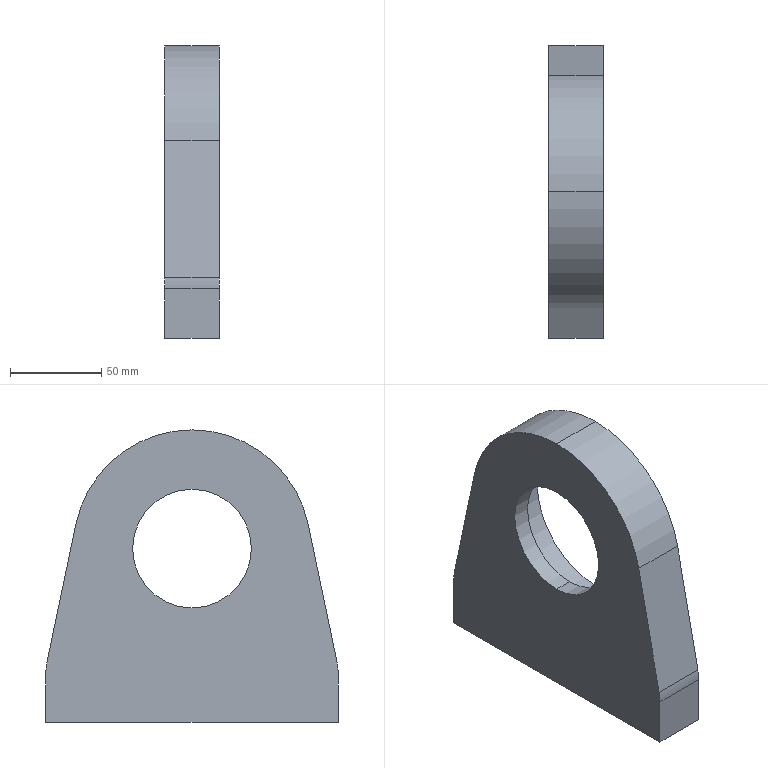Part | SolidWorks | features BaseBody 1 | 1 solid | 16 faces | box 30 x 160 x 160 mm | volume 468530 mm3 | cylinder 8 | plane 8 | commonest cylinder face diameters 60 x2 65 x2 90 x2 130 x2
STEP:
#1=CARTESIAN_POINT('',(10.,0.,60.));
#2=VERTEX_POINT('',#1);
#3=CARTESIAN_POINT('',(10.,0.,-30.));
#4=VERTEX_POINT('',#3);
#5=CARTESIAN_POINT('',(10.,0.,15.));
#6=DIRECTION('',(1.,0.,0.));
#7=DIRECTION('',(0.,0.,-1.));
#8=AXIS2_PLACEMENT_3D('',#5,#6,#7);
#9=CIRCLE('',#8,45.);
#10=EDGE_CURVE('',#2,#4,#9,.T.);
#11=ORIENTED_EDGE('',*,*,#10,.F.);
#12=CARTESIAN_POINT('',(30.,0.,60.));
#13=VERTEX_POINT('',#12);
#14=CARTESIAN_POINT('',(10.,0.,60.));
#15=DIRECTION('',(1.,0.,0.));
#16=VECTOR('',#15,1000.);
#17=LINE('',#14,#16);
#18=EDGE_CURVE('',#2,#13,#17,.T.);
#19=ORIENTED_EDGE('',*,*,#18,.T.);
#20=CARTESIAN_POINT('',(30.,0.,-30.));
#21=VERTEX_POINT('',#20);
#22=CARTESIAN_POINT('',(30.,0.,15.));
#23=DIRECTION('',(1.,0.,0.));
#24=DIRECTION('',(0.,0.,-1.));
#25=AXIS2_PLACEMENT_3D('',#22,#23,#24);
#26=CIRCLE('',#25,45.);
#27=EDGE_CURVE('',#13,#21,#26,.T.);
#28=ORIENTED_EDGE('',*,*,#27,.T.);
#29=CARTESIAN_POINT('',(10.,0.,-30.));
#30=DIRECTION('',(1.,0.,0.));
#31=VECTOR('',#30,1000.);
#32=LINE('',#29,#31);
#33=EDGE_CURVE('',#4,#21,#32,.T.);
#34=ORIENTED_EDGE('',*,*,#33,.F.);
#35=EDGE_LOOP('',(#11,#19,#28,#34));
#36=FACE_OUTER_BOUND('',#35,.T.);
#37=CARTESIAN_POINT('',(10.,0.,15.));
#38=DIRECTION('',(1.,0.,0.));
#39=DIRECTION('',(0.,0.,-1.));
#40=AXIS2_PLACEMENT_3D('',#37,#38,#39);
#41=CYLINDRICAL_SURFACE('',#40,45.);
#42=ADVANCED_FACE('',(#36),#41,.F.);
#43=CARTESIAN_POINT('',(30.,0.,80.));
#44=VERTEX_POINT('',#43);
#45=CARTESIAN_POINT('',(30.,-63.624,28.306));
#46=VERTEX_POINT('',#45);
#47=CARTESIAN_POINT('',(30.,0.,15.));
#48=DIRECTION('',(1.,0.,0.));
#49=DIRECTION('',(0.,0.,-1.));
#50=AXIS2_PLACEMENT_3D('',#47,#48,#49);
#51=CIRCLE('',#50,65.);
#52=EDGE_CURVE('',#44,#46,#51,.T.);
#53=ORIENTED_EDGE('',*,*,#52,.F.);
#54=CARTESIAN_POINT('',(0.,0.,80.));
#55=VERTEX_POINT('',#54);
#56=CARTESIAN_POINT('',(30.,0.,80.));
#57=DIRECTION('',(-1.,0.,0.));
#58=VECTOR('',#57,1000.);
#59=LINE('',#56,#58);
#60=EDGE_CURVE('',#44,#55,#59,.T.);
#61=ORIENTED_EDGE('',*,*,#60,.T.);
#62=CARTESIAN_POINT('',(0.,-63.624,28.306));
#63=VERTEX_POINT('',#62);
#64=CARTESIAN_POINT('',(0.,0.,15.));
#65=DIRECTION('',(1.,0.,0.));
#66=DIRECTION('',(0.,0.,-1.));
#67=AXIS2_PLACEMENT_3D('',#64,#65,#66);
#68=CIRCLE('',#67,65.);
#69=EDGE_CURVE('',#55,#63,#68,.T.);
#70=ORIENTED_EDGE('',*,*,#69,.T.);
#71=CARTESIAN_POINT('',(30.,-63.624,28.306));
#72=DIRECTION('',(-1.,0.,0.));
#73=VECTOR('',#72,1000.);
#74=LINE('',#71,#73);
#75=EDGE_CURVE('',#46,#63,#74,.T.);
#76=ORIENTED_EDGE('',*,*,#75,.F.);
#77=EDGE_LOOP('',(#53,#61,#70,#76));
#78=FACE_OUTER_BOUND('',#77,.T.);
#79=CARTESIAN_POINT('',(30.,0.,15.));
#80=DIRECTION('',(-1.,0.,0.));
#81=DIRECTION('',(0.,0.,1.));
#82=AXIS2_PLACEMENT_3D('',#79,#80,#81);
#83=CYLINDRICAL_SURFACE('',#82,65.);
#84=ADVANCED_FACE('',(#78),#83,.T.);
#85=CARTESIAN_POINT('',(10.,0.,47.5));
#86=VERTEX_POINT('',#85);
#87=CARTESIAN_POINT('',(10.,0.,-17.5));
#88=VERTEX_POINT('',#87);
#89=CARTESIAN_POINT('',(10.,0.,15.));
#90=DIRECTION('',(1.,0.,0.));
#91=DIRECTION('',(0.,0.,-1.));
#92=AXIS2_PLACEMENT_3D('',#89,#90,#91);
#93=CIRCLE('',#92,32.5);
#94=EDGE_CURVE('',#86,#88,#93,.T.);
#95=ORIENTED_EDGE('',*,*,#94,.T.);
#96=CARTESIAN_POINT('',(0.,0.,-17.5));
#97=VERTEX_POINT('',#96);
#98=CARTESIAN_POINT('',(30.,0.,-17.5));
#99=DIRECTION('',(-1.,0.,0.));
#100=VECTOR('',#99,1000.);
#101=LINE('',#98,#100);
#102=EDGE_CURVE('',#88,#97,#101,.T.);
#103=ORIENTED_EDGE('',*,*,#102,.T.);
#104=CARTESIAN_POINT('',(0.,0.,47.5));
#105=VERTEX_POINT('',#104);
#106=CARTESIAN_POINT('',(0.,0.,15.));
#107=DIRECTION('',(1.,0.,0.));
#108=DIRECTION('',(0.,0.,-1.));
#109=AXIS2_PLACEMENT_3D('',#106,#107,#108);
#110=CIRCLE('',#109,32.5);
#111=EDGE_CURVE('',#105,#97,#110,.T.);
#112=ORIENTED_EDGE('',*,*,#111,.F.);
#113=CARTESIAN_POINT('',(30.,0.,47.5));
#114=DIRECTION('',(-1.,0.,0.));
#115=VECTOR('',#114,1000.);
#116=LINE('',#113,#115);
#117=EDGE_CURVE('',#86,#105,#116,.T.);
#118=ORIENTED_EDGE('',*,*,#117,.F.);
#119=EDGE_LOOP('',(#95,#103,#112,#118));
#120=FACE_OUTER_BOUND('',#119,.T.);
#121=CARTESIAN_POINT('',(30.,0.,15.));
#122=DIRECTION('',(-1.,0.,0.));
#123=DIRECTION('',(0.,0.,1.));
#124=AXIS2_PLACEMENT_3D('',#121,#122,#123);
#125=CYLINDRICAL_SURFACE('',#124,32.5);
#126=ADVANCED_FACE('',(#120),#125,.F.);
#127=ORIENTED_EDGE('',*,*,#102,.F.);
#128=CARTESIAN_POINT('',(10.,0.,15.));
#129=DIRECTION('',(1.,0.,0.));
#130=DIRECTION('',(0.,0.,-1.));
#131=AXIS2_PLACEMENT_3D('',#128,#129,#130);
#132=CIRCLE('',#131,32.5);
#133=EDGE_CURVE('',#88,#86,#132,.T.);
#134=ORIENTED_EDGE('',*,*,#133,.T.);
#135=ORIENTED_EDGE('',*,*,#117,.T.);
#136=CARTESIAN_POINT('',(0.,0.,15.));
#137=DIRECTION('',(1.,0.,0.));
#138=DIRECTION('',(0.,0.,-1.));
#139=AXIS2_PLACEMENT_3D('',#136,#137,#138);
#140=CIRCLE('',#139,32.5);
#141=EDGE_CURVE('',#97,#105,#140,.T.);
#142=ORIENTED_EDGE('',*,*,#141,.F.);
#143=EDGE_LOOP('',(#127,#134,#135,#142));
#144=FACE_OUTER_BOUND('',#143,.T.);
#145=CARTESIAN_POINT('',(30.,0.,15.));
#146=DIRECTION('',(-1.,0.,0.));
#147=DIRECTION('',(0.,0.,1.));
#148=AXIS2_PLACEMENT_3D('',#145,#146,#147);
#149=CYLINDRICAL_SURFACE('',#148,32.5);
#150=ADVANCED_FACE('',(#144),#149,.F.);
#151=CARTESIAN_POINT('',(30.,0.,15.));
#152=DIRECTION('',(1.,0.,0.));
#153=DIRECTION('',(0.,0.,-1.));
#154=AXIS2_PLACEMENT_3D('',#151,#152,#153);
#155=CIRCLE('',#154,45.);
#156=EDGE_CURVE('',#21,#13,#155,.T.);
#157=ORIENTED_EDGE('',*,*,#156,.F.);
#158=ORIENTED_EDGE('',*,*,#27,.F.);
#159=EDGE_LOOP('',(#157,#158));
#160=FACE_BOUND('',#159,.T.);
#161=CARTESIAN_POINT('',(30.,80.,-80.));
#162=VERTEX_POINT('',#161);
#163=CARTESIAN_POINT('',(30.,80.,-53.103));
#164=VERTEX_POINT('',#163);
#165=CARTESIAN_POINT('',(30.,80.,-80.));
#166=DIRECTION('',(0.,0.,1.));
#167=VECTOR('',#166,1000.);
#168=LINE('',#165,#167);
#169=EDGE_CURVE('',#162,#164,#168,.T.);
#170=ORIENTED_EDGE('',*,*,#169,.T.);
#171=CARTESIAN_POINT('',(30.,79.365,-46.962));
#172=VERTEX_POINT('',#171);
#173=CARTESIAN_POINT('',(30.,50.,-53.103));
#174=DIRECTION('',(1.,0.,0.));
#175=DIRECTION('',(0.,0.,1.));
#176=AXIS2_PLACEMENT_3D('',#173,#174,#175);
#177=CIRCLE('',#176,30.);
#178=EDGE_CURVE('',#164,#172,#177,.T.);
#179=ORIENTED_EDGE('',*,*,#178,.T.);
#180=CARTESIAN_POINT('',(30.,63.624,28.306));
#181=VERTEX_POINT('',#180);
#182=CARTESIAN_POINT('',(30.,79.365,-46.962));
#183=DIRECTION('',(0.,-0.2047,0.9788));
#184=VECTOR('',#183,1000.);
#185=LINE('',#182,#184);
#186=EDGE_CURVE('',#172,#181,#185,.T.);
#187=ORIENTED_EDGE('',*,*,#186,.T.);
#188=CARTESIAN_POINT('',(30.,0.,15.));
#189=DIRECTION('',(1.,0.,0.));
#190=DIRECTION('',(0.,0.,-1.));
#191=AXIS2_PLACEMENT_3D('',#188,#189,#190);
#192=CIRCLE('',#191,65.);
#193=EDGE_CURVE('',#181,#44,#192,.T.);
#194=ORIENTED_EDGE('',*,*,#193,.T.);
#195=ORIENTED_EDGE('',*,*,#52,.T.);
#196=CARTESIAN_POINT('',(30.,-79.365,-46.962));
#197=VERTEX_POINT('',#196);
#198=CARTESIAN_POINT('',(30.,-79.365,-46.962));
#199=DIRECTION('',(0.,-0.2047,-0.9788));
#200=VECTOR('',#199,1000.);
#201=LINE('',#198,#200);
#202=EDGE_CURVE('',#46,#197,#201,.T.);
#203=ORIENTED_EDGE('',*,*,#202,.T.);
#204=CARTESIAN_POINT('',(30.,-80.,-53.103));
#205=VERTEX_POINT('',#204);
#206=CARTESIAN_POINT('',(30.,-50.,-53.103));
#207=DIRECTION('',(1.,0.,0.));
#208=DIRECTION('',(0.,0.,-1.));
#209=AXIS2_PLACEMENT_3D('',#206,#207,#208);
#210=CIRCLE('',#209,30.);
#211=EDGE_CURVE('',#197,#205,#210,.T.);
#212=ORIENTED_EDGE('',*,*,#211,.T.);
#213=CARTESIAN_POINT('',(30.,-80.,-80.));
#214=VERTEX_POINT('',#213);
#215=CARTESIAN_POINT('',(30.,-80.,-80.));
#216=DIRECTION('',(0.,0.,-1.));
#217=VECTOR('',#216,1000.);
#218=LINE('',#215,#217);
#219=EDGE_CURVE('',#205,#214,#218,.T.);
#220=ORIENTED_EDGE('',*,*,#219,.T.);
#221=CARTESIAN_POINT('',(30.,80.,-80.));
#222=DIRECTION('',(0.,1.,0.));
#223=VECTOR('',#222,1000.);
#224=LINE('',#221,#223);
#225=EDGE_CURVE('',#214,#162,#224,.T.);
#226=ORIENTED_EDGE('',*,*,#225,.T.);
#227=EDGE_LOOP('',(#170,#179,#187,#194,#195,#203,#212,#220,#226));
#228=FACE_OUTER_BOUND('',#227,.T.);
#229=CARTESIAN_POINT('',(30.,50.,-53.103));
#230=DIRECTION('',(-1.,0.,0.));
#231=DIRECTION('',(0.,0.,1.));
#232=AXIS2_PLACEMENT_3D('',#229,#230,#231);
#233=PLANE('',#232);
#234=ADVANCED_FACE('',(#160,#228),#233,.F.);
#235=CARTESIAN_POINT('',(0.,80.,-80.));
#236=VERTEX_POINT('',#235);
#237=CARTESIAN_POINT('',(0.,80.,-53.103));
#238=VERTEX_POINT('',#237);
#239=CARTESIAN_POINT('',(0.,80.,-80.));
#240=DIRECTION('',(0.,0.,1.));
#241=VECTOR('',#240,1000.);
#242=LINE('',#239,#241);
#243=EDGE_CURVE('',#236,#238,#242,.T.);
#244=ORIENTED_EDGE('',*,*,#243,.F.);
#245=CARTESIAN_POINT('',(0.,-80.,-80.));
#246=VERTEX_POINT('',#245);
#247=CARTESIAN_POINT('',(0.,80.,-80.));
#248=DIRECTION('',(0.,1.,0.));
#249=VECTOR('',#248,1000.);
#250=LINE('',#247,#249);
#251=EDGE_CURVE('',#246,#236,#250,.T.);
#252=ORIENTED_EDGE('',*,*,#251,.F.);
#253=CARTESIAN_POINT('',(0.,-80.,-53.103));
#254=VERTEX_POINT('',#253);
#255=CARTESIAN_POINT('',(0.,-80.,-80.));
#256=DIRECTION('',(0.,0.,-1.));
#257=VECTOR('',#256,1000.);
#258=LINE('',#255,#257);
#259=EDGE_CURVE('',#254,#246,#258,.T.);
#260=ORIENTED_EDGE('',*,*,#259,.F.);
#261=CARTESIAN_POINT('',(0.,-79.365,-46.962));
#262=VERTEX_POINT('',#261);
#263=CARTESIAN_POINT('',(0.,-50.,-53.103));
#264=DIRECTION('',(1.,0.,0.));
#265=DIRECTION('',(0.,0.,-1.));
#266=AXIS2_PLACEMENT_3D('',#263,#264,#265);
#267=CIRCLE('',#266,30.);
#268=EDGE_CURVE('',#262,#254,#267,.T.);
#269=ORIENTED_EDGE('',*,*,#268,.F.);
#270=CARTESIAN_POINT('',(0.,-79.365,-46.962));
#271=DIRECTION('',(0.,-0.2047,-0.9788));
#272=VECTOR('',#271,1000.);
#273=LINE('',#270,#272);
#274=EDGE_CURVE('',#63,#262,#273,.T.);
#275=ORIENTED_EDGE('',*,*,#274,.F.);
#276=ORIENTED_EDGE('',*,*,#69,.F.);
#277=CARTESIAN_POINT('',(0.,63.624,28.306));
#278=VERTEX_POINT('',#277);
#279=CARTESIAN_POINT('',(0.,0.,15.));
#280=DIRECTION('',(1.,0.,0.));
#281=DIRECTION('',(0.,0.,-1.));
#282=AXIS2_PLACEMENT_3D('',#279,#280,#281);
#283=CIRCLE('',#282,65.);
#284=EDGE_CURVE('',#278,#55,#283,.T.);
#285=ORIENTED_EDGE('',*,*,#284,.F.);
#286=CARTESIAN_POINT('',(0.,79.365,-46.962));
#287=VERTEX_POINT('',#286);
#288=CARTESIAN_POINT('',(0.,79.365,-46.962));
#289=DIRECTION('',(0.,-0.2047,0.9788));
#290=VECTOR('',#289,1000.);
#291=LINE('',#288,#290);
#292=EDGE_CURVE('',#287,#278,#291,.T.);
#293=ORIENTED_EDGE('',*,*,#292,.F.);
#294=CARTESIAN_POINT('',(0.,50.,-53.103));
#295=DIRECTION('',(1.,0.,0.));
#296=DIRECTION('',(0.,0.,1.));
#297=AXIS2_PLACEMENT_3D('',#294,#295,#296);
#298=CIRCLE('',#297,30.);
#299=EDGE_CURVE('',#238,#287,#298,.T.);
#300=ORIENTED_EDGE('',*,*,#299,.F.);
#301=EDGE_LOOP('',(#244,#252,#260,#269,#275,#276,#285,#293,#300));
#302=FACE_OUTER_BOUND('',#301,.T.);
#303=ORIENTED_EDGE('',*,*,#111,.T.);
#304=ORIENTED_EDGE('',*,*,#141,.T.);
#305=EDGE_LOOP('',(#303,#304));
#306=FACE_BOUND('',#305,.T.);
#307=CARTESIAN_POINT('',(0.,50.,-53.103));
#308=DIRECTION('',(-1.,0.,0.));
#309=DIRECTION('',(0.,0.,1.));
#310=AXIS2_PLACEMENT_3D('',#307,#308,#309);
#311=PLANE('',#310);
#312=ADVANCED_FACE('',(#302,#306),#311,.T.);
#313=ORIENTED_EDGE('',*,*,#243,.T.);
#314=CARTESIAN_POINT('',(30.,80.,-53.103));
#315=DIRECTION('',(-1.,0.,0.));
#316=VECTOR('',#315,1000.);
#317=LINE('',#314,#316);
#318=EDGE_CURVE('',#164,#238,#317,.T.);
#319=ORIENTED_EDGE('',*,*,#318,.F.);
#320=ORIENTED_EDGE('',*,*,#169,.F.);
#321=CARTESIAN_POINT('',(30.,80.,-80.));
#322=DIRECTION('',(-1.,0.,0.));
#323=VECTOR('',#322,1000.);
#324=LINE('',#321,#323);
#325=EDGE_CURVE('',#162,#236,#324,.T.);
#326=ORIENTED_EDGE('',*,*,#325,.T.);
#327=EDGE_LOOP('',(#313,#319,#320,#326));
#328=FACE_OUTER_BOUND('',#327,.T.);
#329=CARTESIAN_POINT('',(30.,80.,-80.));
#330=DIRECTION('',(0.,-1.,0.));
#331=DIRECTION('',(0.,0.,-1.));
#332=AXIS2_PLACEMENT_3D('',#329,#330,#331);
#333=PLANE('',#332);
#334=ADVANCED_FACE('',(#328),#333,.F.);
#335=ORIENTED_EDGE('',*,*,#299,.T.);
#336=CARTESIAN_POINT('',(30.,79.365,-46.962));
#337=DIRECTION('',(-1.,0.,0.));
#338=VECTOR('',#337,1000.);
#339=LINE('',#336,#338);
#340=EDGE_CURVE('',#172,#287,#339,.T.);
#341=ORIENTED_EDGE('',*,*,#340,.F.);
#342=ORIENTED_EDGE('',*,*,#178,.F.);
#343=ORIENTED_EDGE('',*,*,#318,.T.);
#344=EDGE_LOOP('',(#335,#341,#342,#343));
#345=FACE_OUTER_BOUND('',#344,.T.);
#346=CARTESIAN_POINT('',(30.,50.,-53.103));
#347=DIRECTION('',(-1.,0.,0.));
#348=DIRECTION('',(0.,0.,1.));
#349=AXIS2_PLACEMENT_3D('',#346,#347,#348);
#350=CYLINDRICAL_SURFACE('',#349,30.);
#351=ADVANCED_FACE('',(#345),#350,.T.);
#352=ORIENTED_EDGE('',*,*,#292,.T.);
#353=CARTESIAN_POINT('',(30.,63.624,28.306));
#354=DIRECTION('',(-1.,0.,0.));
#355=VECTOR('',#354,1000.);
#356=LINE('',#353,#355);
#357=EDGE_CURVE('',#181,#278,#356,.T.);
#358=ORIENTED_EDGE('',*,*,#357,.F.);
#359=ORIENTED_EDGE('',*,*,#186,.F.);
#360=ORIENTED_EDGE('',*,*,#340,.T.);
#361=EDGE_LOOP('',(#352,#358,#359,#360));
#362=FACE_OUTER_BOUND('',#361,.T.);
#363=CARTESIAN_POINT('',(30.,79.365,-46.962));
#364=DIRECTION('',(0.,-0.9788,-0.2047));
#365=DIRECTION('',(0.,0.2047,-0.9788));
#366=AXIS2_PLACEMENT_3D('',#363,#364,#365);
#367=PLANE('',#366);
#368=ADVANCED_FACE('',(#362),#367,.F.);
#369=ORIENTED_EDGE('',*,*,#60,.F.);
#370=ORIENTED_EDGE('',*,*,#193,.F.);
#371=ORIENTED_EDGE('',*,*,#357,.T.);
#372=ORIENTED_EDGE('',*,*,#284,.T.);
#373=EDGE_LOOP('',(#369,#370,#371,#372));
#374=FACE_OUTER_BOUND('',#373,.T.);
#375=CARTESIAN_POINT('',(30.,0.,15.));
#376=DIRECTION('',(-1.,0.,0.));
#377=DIRECTION('',(0.,0.,1.));
#378=AXIS2_PLACEMENT_3D('',#375,#376,#377);
#379=CYLINDRICAL_SURFACE('',#378,65.);
#380=ADVANCED_FACE('',(#374),#379,.T.);
#381=ORIENTED_EDGE('',*,*,#274,.T.);
#382=CARTESIAN_POINT('',(30.,-79.365,-46.962));
#383=DIRECTION('',(-1.,0.,0.));
#384=VECTOR('',#383,1000.);
#385=LINE('',#382,#384);
#386=EDGE_CURVE('',#197,#262,#385,.T.);
#387=ORIENTED_EDGE('',*,*,#386,.F.);
#388=ORIENTED_EDGE('',*,*,#202,.F.);
#389=ORIENTED_EDGE('',*,*,#75,.T.);
#390=EDGE_LOOP('',(#381,#387,#388,#389));
#391=FACE_OUTER_BOUND('',#390,.T.);
#392=CARTESIAN_POINT('',(30.,-79.365,-46.962));
#393=DIRECTION('',(0.,0.9788,-0.2047));
#394=DIRECTION('',(0.,0.2047,0.9788));
#395=AXIS2_PLACEMENT_3D('',#392,#393,#394);
#396=PLANE('',#395);
#397=ADVANCED_FACE('',(#391),#396,.F.);
#398=ORIENTED_EDGE('',*,*,#268,.T.);
#399=CARTESIAN_POINT('',(30.,-80.,-53.103));
#400=DIRECTION('',(-1.,0.,0.));
#401=VECTOR('',#400,1000.);
#402=LINE('',#399,#401);
#403=EDGE_CURVE('',#205,#254,#402,.T.);
#404=ORIENTED_EDGE('',*,*,#403,.F.);
#405=ORIENTED_EDGE('',*,*,#211,.F.);
#406=ORIENTED_EDGE('',*,*,#386,.T.);
#407=EDGE_LOOP('',(#398,#404,#405,#406));
#408=FACE_OUTER_BOUND('',#407,.T.);
#409=CARTESIAN_POINT('',(30.,-50.,-53.103));
#410=DIRECTION('',(-1.,0.,0.));
#411=DIRECTION('',(0.,0.,1.));
#412=AXIS2_PLACEMENT_3D('',#409,#410,#411);
#413=CYLINDRICAL_SURFACE('',#412,30.);
#414=ADVANCED_FACE('',(#408),#413,.T.);
#415=ORIENTED_EDGE('',*,*,#259,.T.);
#416=CARTESIAN_POINT('',(30.,-80.,-80.));
#417=DIRECTION('',(-1.,0.,0.));
#418=VECTOR('',#417,1000.);
#419=LINE('',#416,#418);
#420=EDGE_CURVE('',#214,#246,#419,.T.);
#421=ORIENTED_EDGE('',*,*,#420,.F.);
#422=ORIENTED_EDGE('',*,*,#219,.F.);
#423=ORIENTED_EDGE('',*,*,#403,.T.);
#424=EDGE_LOOP('',(#415,#421,#422,#423));
#425=FACE_OUTER_BOUND('',#424,.T.);
#426=CARTESIAN_POINT('',(30.,-80.,-80.));
#427=DIRECTION('',(0.,1.,0.));
#428=DIRECTION('',(0.,0.,1.));
#429=AXIS2_PLACEMENT_3D('',#426,#427,#428);
#430=PLANE('',#429);
#431=ADVANCED_FACE('',(#425),#430,.F.);
#432=ORIENTED_EDGE('',*,*,#251,.T.);
#433=ORIENTED_EDGE('',*,*,#325,.F.);
#434=ORIENTED_EDGE('',*,*,#225,.F.);
#435=ORIENTED_EDGE('',*,*,#420,.T.);
#436=EDGE_LOOP('',(#432,#433,#434,#435));
#437=FACE_OUTER_BOUND('',#436,.T.);
#438=CARTESIAN_POINT('',(30.,80.,-80.));
#439=DIRECTION('',(0.,0.,1.));
#440=DIRECTION('',(1.,0.,0.));
#441=AXIS2_PLACEMENT_3D('',#438,#439,#440);
#442=PLANE('',#441);
#443=ADVANCED_FACE('',(#437),#442,.F.);
#444=ORIENTED_EDGE('',*,*,#18,.F.);
#445=CARTESIAN_POINT('',(10.,0.,15.));
#446=DIRECTION('',(1.,0.,0.));
#447=DIRECTION('',(0.,0.,-1.));
#448=AXIS2_PLACEMENT_3D('',#445,#446,#447);
#449=CIRCLE('',#448,45.);
#450=EDGE_CURVE('',#4,#2,#449,.T.);
#451=ORIENTED_EDGE('',*,*,#450,.F.);
#452=ORIENTED_EDGE('',*,*,#33,.T.);
#453=ORIENTED_EDGE('',*,*,#156,.T.);
#454=EDGE_LOOP('',(#444,#451,#452,#453));
#455=FACE_OUTER_BOUND('',#454,.T.);
#456=CARTESIAN_POINT('',(10.,0.,15.));
#457=DIRECTION('',(1.,0.,0.));
#458=DIRECTION('',(0.,0.,-1.));
#459=AXIS2_PLACEMENT_3D('',#456,#457,#458);
#460=CYLINDRICAL_SURFACE('',#459,45.);
#461=ADVANCED_FACE('',(#455),#460,.F.);
#462=ORIENTED_EDGE('',*,*,#94,.F.);
#463=ORIENTED_EDGE('',*,*,#133,.F.);
#464=EDGE_LOOP('',(#462,#463));
#465=FACE_BOUND('',#464,.T.);
#466=ORIENTED_EDGE('',*,*,#450,.T.);
#467=ORIENTED_EDGE('',*,*,#10,.T.);
#468=EDGE_LOOP('',(#466,#467));
#469=FACE_OUTER_BOUND('',#468,.T.);
#470=CARTESIAN_POINT('',(10.,0.,15.));
#471=DIRECTION('',(1.,0.,0.));
#472=DIRECTION('',(0.,0.,-1.));
#473=AXIS2_PLACEMENT_3D('',#470,#471,#472);
#474=PLANE('',#473);
#475=ADVANCED_FACE('',(#465,#469),#474,.T.);
#476=CLOSED_SHELL('',(#42,#84,#126,#150,#234,#312,#334,#351,#368,#380,#397,#414,#431,#443,#461,#475));
#477=MANIFOLD_SOLID_BREP('',#476);
#478=CARTESIAN_POINT('',(0.,0.,0.));
#479=DIRECTION('',(0.,0.,1.));
#480=DIRECTION('',(1.,0.,0.));
#481=AXIS2_PLACEMENT_3D('',#478,#479,#480);
#482=(LENGTH_UNIT()NAMED_UNIT(*)SI_UNIT(.MILLI.,.METRE.));
#483=UNCERTAINTY_MEASURE_WITH_UNIT(LENGTH_MEASURE(0.00001),#482,'','');
#484=(NAMED_UNIT(*)PLANE_ANGLE_UNIT()SI_UNIT($,.RADIAN.));
#485=(NAMED_UNIT(*)SI_UNIT($,.STERADIAN.)SOLID_ANGLE_UNIT());
#486=(GEOMETRIC_REPRESENTATION_CONTEXT(3)GLOBAL_UNCERTAINTY_ASSIGNED_CONTEXT((#483))GLOBAL_UNIT_ASSIGNED_CONTEXT((#482,#484,#485))REPRESENTATION_CONTEXT('',''));
#487=ADVANCED_BREP_SHAPE_REPRESENTATION('',(#477,#481),#486);